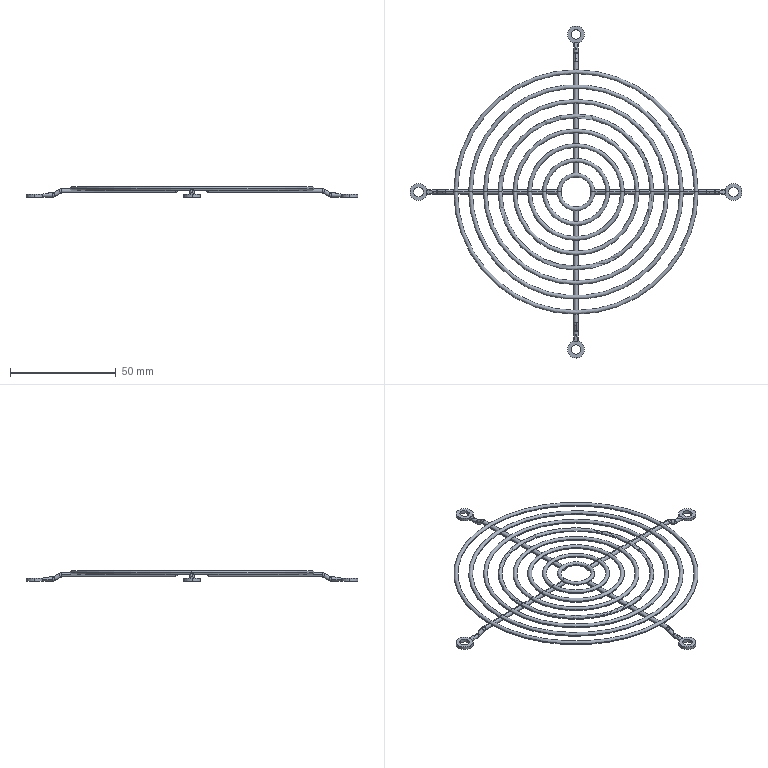Part | SolidWorks | features ICE 4, Fillet 2, CirPattern 1, RefAxis 1, Revolution 1, Sweep 1 | 4 solids | 121 faces | box 157.05 x 157.05 x 4.9 mm | volume 5119 mm3 | torus 56 | cylinder 48 | plane 12 | sphere 5 | commonest cylinder face diameters 2 x24 8 x16 4.5 x8